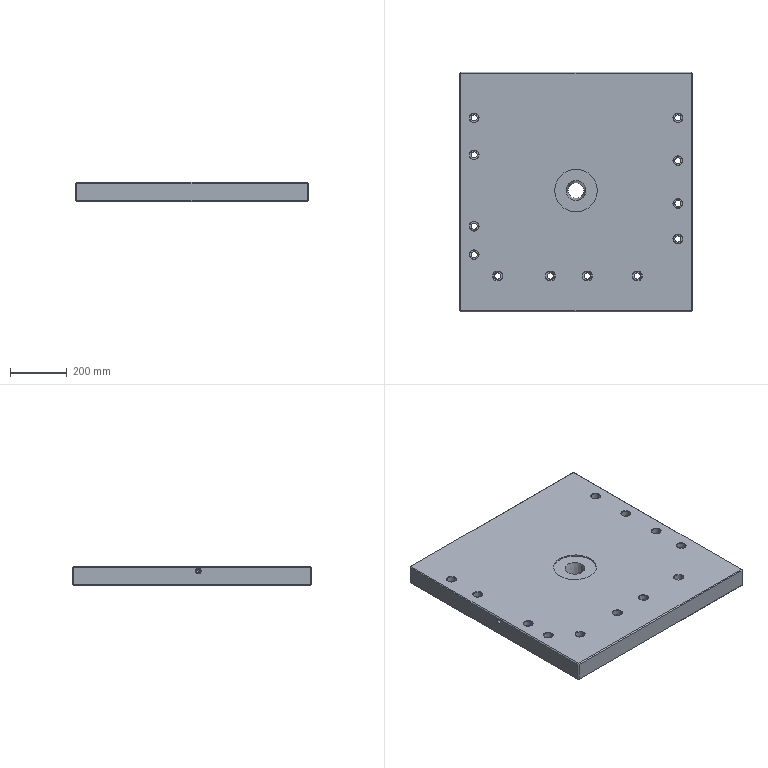Part | Creo | 1 solid | 189 faces | box 815 x 840 x 70 mm | volume 44062103 mm3 | cone 66 | cylinder 64 | plane 59 | commonest cylinder face diameters 21.5 x16 31.5 x16 32 x12 22 x8 28 x4 14 x2